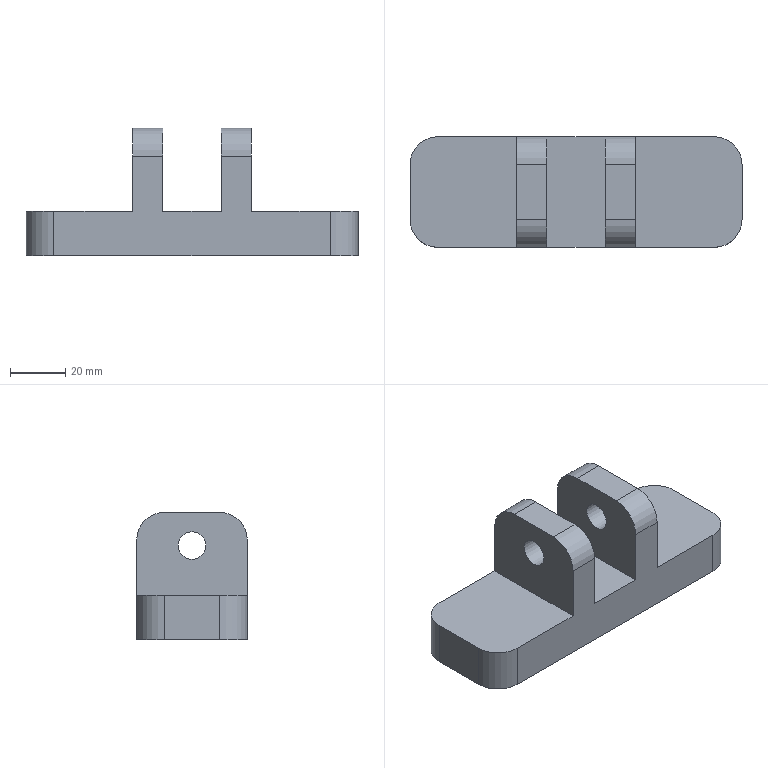CAM job | NX | 3+2 milling, drilling | part box 120 x 40 x 46 mm | stock box 127 x 50 x 50 mm
Tools:
number,name,description,diameter,corner_radius,flute_length,length,flutes
1,D50面刀,Milling Tool-5 Parameters,50.0,0.0,50.0,75.0,2
2,D16开粗,Milling Tool-5 Parameters,16.0,0.0,50.0,75.0,2
3,D16精光,Milling Tool-5 Parameters,16.0,0.0,50.0,75.0,2
4,D6R0.5,Milling Tool-5 Parameters,6.0,0.5,50.0,75.0,2
5,D6倒角刀,Milling Tool-5 Parameters,6.0,0.0,50.0,75.0,2
10,D10钻头,Drilling Tool,10.0,0.0,35.0,50.0,2
Operations:
program,operation,operation_type,tool,method,geometry_group,spindle_rpm,surface_speed,feed_per_tooth,feed_cut,feed_plunge,cut_length_mm,path_length_mm,cut_time_min,machine_time_min
G54,PLANAR_MILL,PlanarMilling,D50面刀,METHOD,WORKPIECE,1600.0,251.0,0.1875,600.0,100.0,164.0,200.0,0.2733,0.2769
G54,ADAPTIVE_MILLING,CavityMilling,D16开粗,METHOD,WORKPIECE,4500.0,226.0,0.3333,3000.0,100.0,60516.141,64043.105,15.156,15.509
G54,ADAPTIVE_MILLING_COPY,CavityMilling,D16开粗,METHOD,WORKPIECE,4500.0,226.0,0.3333,3000.0,100.0,10032.027,10160.027,2.809,2.821
G54,FLOOR_FACING,VolumeBased25DMillingOperation,D16精光,METHOD,WORKPIECE,2200.0,110.0,0.1364,600.0,100.0,650.421,1119.035,1.084,1.131
G54,PLANAR_MILL_1_COPY,PlanarMilling,D16精光,METHOD,WORKPIECE,2200.0,110.0,0.1364,600.0,100.0,528.0,1603.066,0.88,0.9875
G54,PLANAR_MILL_1,PlanarMilling,D16精光,METHOD,WORKPIECE,2200.0,110.0,0.1364,600.0,100.0,730.414,860.414,1.217,1.23
G54,ZLEVEL_PROFILE_STEEP,ZLevelMilling,D6R0.5,METHOD,WORKPIECE,3000.0,56.0,0.25,1500.0,100.0,9339.794,9668.152,6.226,6.259
G54,PLANAR_MILL_2,PlanarMilling,D6倒角刀,METHOD,WORKPIECE,3000.0,56.0,0.1333,800.0,100.0,128.0,335.0,0.16,0.1807
G54,PLANAR_MILL_3,PlanarMilling,D6倒角刀,METHOD,WORKPIECE,3000.0,56.0,0.1333,800.0,100.0,287.331,727.231,0.3592,0.4032
G55,PLANAR_MILL_4,PlanarMilling,D50面刀,METHOD,G55,1600.0,251.0,0.1875,600.0,100.0,206.0,240.0,0.3433,0.3467
G55,PLANAR_MILL_5,PlanarMilling,D6倒角刀,METHOD,G55,3000.0,56.0,0.1,600.0,100.0,325.681,365.681,0.5428,0.5468
G56,DRILLING,Operation,D6倒角刀,METHOD,G56,0.0,0.0,0.0,250.0,0.0,4.5,126.0,0.018,0.0301
G56,DRILLING_COPY,Operation,D10钻头,METHOD,G56,800.0,25.0,0.0312,50.0,0.0,18.0,153.0,0.36,0.3735